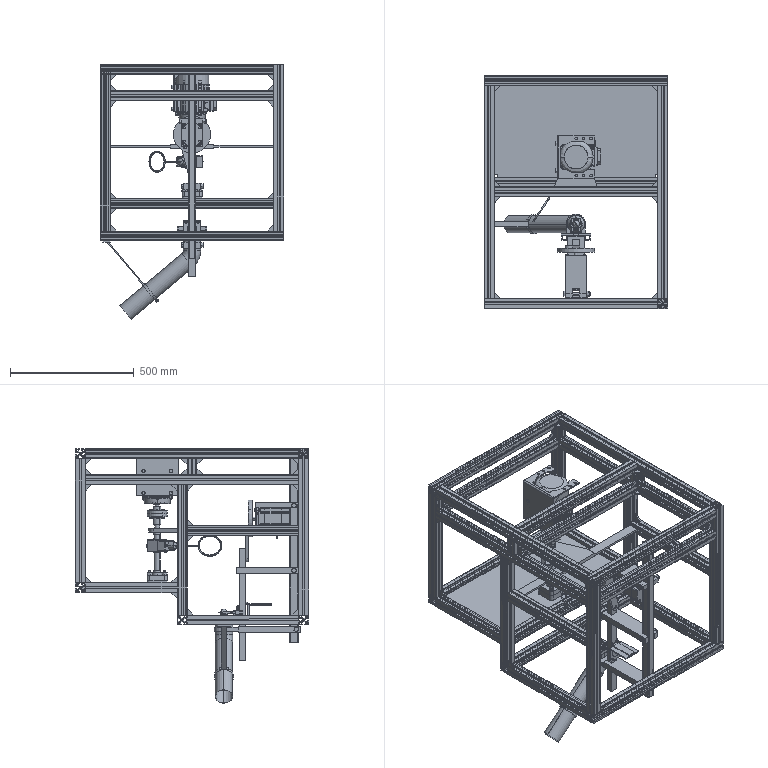Part | SolidWorks | features InContextFeatHolder 17, ReferencePattern 17, MirrorCompFeat 8, CompositeCurve 4, Cut 1, RefAxis 1 | 254 solids | 7090 faces | volume 20823217 mm3 | plane 3795 | cylinder 1609 | cone 1115 | torus 297 | spline 168 | sphere 106 | commonest cylinder face diameters 8 x321 1 x160 2 x124 5 x74 6 x64 6.8 x60